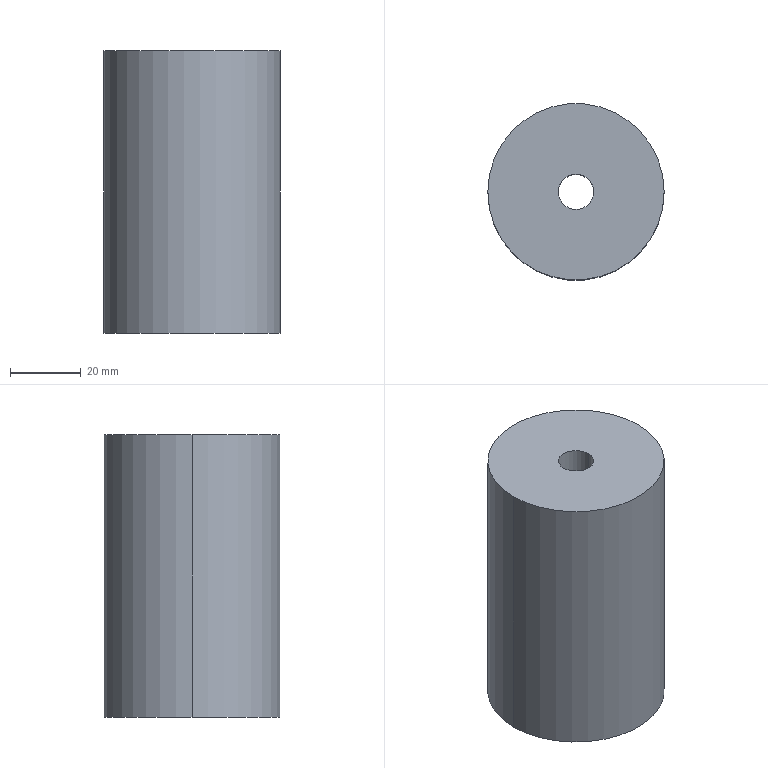Part | SolidWorks | features Extrusion 1 | 1 solid | 6 faces | box 50 x 50 x 80 mm | volume 150796 mm3 | cylinder 4 | plane 2 | commonest cylinder face diameters 10 x2 50 x2
STEP:
#1=CARTESIAN_POINT('',(-5.,0.,80.));
#2=VERTEX_POINT('',#1);
#3=CARTESIAN_POINT('',(5.,0.,80.));
#4=VERTEX_POINT('',#3);
#5=CARTESIAN_POINT('',(0.,0.,80.));
#6=DIRECTION('',(0.,0.,1.));
#7=DIRECTION('',(1.,0.,0.));
#8=AXIS2_PLACEMENT_3D('',#5,#6,#7);
#9=CIRCLE('',#8,5.);
#10=EDGE_CURVE('',#2,#4,#9,.T.);
#11=ORIENTED_EDGE('',*,*,#10,.T.);
#12=CARTESIAN_POINT('',(5.,0.,0.));
#13=VERTEX_POINT('',#12);
#14=CARTESIAN_POINT('',(5.,0.,80.));
#15=DIRECTION('',(0.,0.,-1.));
#16=VECTOR('',#15,1000.);
#17=LINE('',#14,#16);
#18=EDGE_CURVE('',#4,#13,#17,.T.);
#19=ORIENTED_EDGE('',*,*,#18,.T.);
#20=CARTESIAN_POINT('',(-5.,0.,0.));
#21=VERTEX_POINT('',#20);
#22=CARTESIAN_POINT('',(0.,0.,0.));
#23=DIRECTION('',(0.,0.,1.));
#24=DIRECTION('',(1.,0.,0.));
#25=AXIS2_PLACEMENT_3D('',#22,#23,#24);
#26=CIRCLE('',#25,5.);
#27=EDGE_CURVE('',#21,#13,#26,.T.);
#28=ORIENTED_EDGE('',*,*,#27,.F.);
#29=CARTESIAN_POINT('',(-5.,0.,80.));
#30=DIRECTION('',(0.,0.,-1.));
#31=VECTOR('',#30,1000.);
#32=LINE('',#29,#31);
#33=EDGE_CURVE('',#2,#21,#32,.T.);
#34=ORIENTED_EDGE('',*,*,#33,.F.);
#35=EDGE_LOOP('',(#11,#19,#28,#34));
#36=FACE_OUTER_BOUND('',#35,.T.);
#37=CARTESIAN_POINT('',(0.,0.,80.));
#38=DIRECTION('',(0.,0.,-1.));
#39=DIRECTION('',(-1.,0.,0.));
#40=AXIS2_PLACEMENT_3D('',#37,#38,#39);
#41=CYLINDRICAL_SURFACE('',#40,5.);
#42=ADVANCED_FACE('',(#36),#41,.F.);
#43=CARTESIAN_POINT('',(25.,0.,80.));
#44=VERTEX_POINT('',#43);
#45=CARTESIAN_POINT('',(-25.,0.,80.));
#46=VERTEX_POINT('',#45);
#47=CARTESIAN_POINT('',(0.,0.,80.));
#48=DIRECTION('',(0.,0.,1.));
#49=DIRECTION('',(1.,0.,0.));
#50=AXIS2_PLACEMENT_3D('',#47,#48,#49);
#51=CIRCLE('',#50,25.);
#52=EDGE_CURVE('',#44,#46,#51,.T.);
#53=ORIENTED_EDGE('',*,*,#52,.F.);
#54=CARTESIAN_POINT('',(25.,0.,0.));
#55=VERTEX_POINT('',#54);
#56=CARTESIAN_POINT('',(25.,0.,80.));
#57=DIRECTION('',(0.,0.,-1.));
#58=VECTOR('',#57,1000.);
#59=LINE('',#56,#58);
#60=EDGE_CURVE('',#44,#55,#59,.T.);
#61=ORIENTED_EDGE('',*,*,#60,.T.);
#62=CARTESIAN_POINT('',(-25.,0.,0.));
#63=VERTEX_POINT('',#62);
#64=CARTESIAN_POINT('',(0.,0.,0.));
#65=DIRECTION('',(0.,0.,1.));
#66=DIRECTION('',(1.,0.,0.));
#67=AXIS2_PLACEMENT_3D('',#64,#65,#66);
#68=CIRCLE('',#67,25.);
#69=EDGE_CURVE('',#55,#63,#68,.T.);
#70=ORIENTED_EDGE('',*,*,#69,.T.);
#71=CARTESIAN_POINT('',(-25.,0.,80.));
#72=DIRECTION('',(0.,0.,-1.));
#73=VECTOR('',#72,1000.);
#74=LINE('',#71,#73);
#75=EDGE_CURVE('',#46,#63,#74,.T.);
#76=ORIENTED_EDGE('',*,*,#75,.F.);
#77=EDGE_LOOP('',(#53,#61,#70,#76));
#78=FACE_OUTER_BOUND('',#77,.T.);
#79=CARTESIAN_POINT('',(0.,0.,80.));
#80=DIRECTION('',(0.,0.,-1.));
#81=DIRECTION('',(-1.,0.,0.));
#82=AXIS2_PLACEMENT_3D('',#79,#80,#81);
#83=CYLINDRICAL_SURFACE('',#82,25.);
#84=ADVANCED_FACE('',(#78),#83,.T.);
#85=CARTESIAN_POINT('',(0.,0.,80.));
#86=DIRECTION('',(0.,0.,1.));
#87=DIRECTION('',(1.,0.,0.));
#88=AXIS2_PLACEMENT_3D('',#85,#86,#87);
#89=CIRCLE('',#88,25.);
#90=EDGE_CURVE('',#46,#44,#89,.T.);
#91=ORIENTED_EDGE('',*,*,#90,.T.);
#92=ORIENTED_EDGE('',*,*,#52,.T.);
#93=EDGE_LOOP('',(#91,#92));
#94=FACE_OUTER_BOUND('',#93,.T.);
#95=ORIENTED_EDGE('',*,*,#10,.F.);
#96=CARTESIAN_POINT('',(0.,0.,80.));
#97=DIRECTION('',(0.,0.,1.));
#98=DIRECTION('',(1.,0.,0.));
#99=AXIS2_PLACEMENT_3D('',#96,#97,#98);
#100=CIRCLE('',#99,5.);
#101=EDGE_CURVE('',#4,#2,#100,.T.);
#102=ORIENTED_EDGE('',*,*,#101,.F.);
#103=EDGE_LOOP('',(#95,#102));
#104=FACE_BOUND('',#103,.T.);
#105=CARTESIAN_POINT('',(0.,0.,80.));
#106=DIRECTION('',(0.,0.,1.));
#107=DIRECTION('',(1.,0.,0.));
#108=AXIS2_PLACEMENT_3D('',#105,#106,#107);
#109=PLANE('',#108);
#110=ADVANCED_FACE('',(#94,#104),#109,.T.);
#111=CARTESIAN_POINT('',(0.,0.,0.));
#112=DIRECTION('',(0.,0.,1.));
#113=DIRECTION('',(1.,0.,0.));
#114=AXIS2_PLACEMENT_3D('',#111,#112,#113);
#115=CIRCLE('',#114,25.);
#116=EDGE_CURVE('',#63,#55,#115,.T.);
#117=ORIENTED_EDGE('',*,*,#116,.F.);
#118=ORIENTED_EDGE('',*,*,#69,.F.);
#119=EDGE_LOOP('',(#117,#118));
#120=FACE_OUTER_BOUND('',#119,.T.);
#121=ORIENTED_EDGE('',*,*,#27,.T.);
#122=CARTESIAN_POINT('',(0.,0.,0.));
#123=DIRECTION('',(0.,0.,1.));
#124=DIRECTION('',(1.,0.,0.));
#125=AXIS2_PLACEMENT_3D('',#122,#123,#124);
#126=CIRCLE('',#125,5.);
#127=EDGE_CURVE('',#13,#21,#126,.T.);
#128=ORIENTED_EDGE('',*,*,#127,.T.);
#129=EDGE_LOOP('',(#121,#128));
#130=FACE_BOUND('',#129,.T.);
#131=CARTESIAN_POINT('',(0.,0.,0.));
#132=DIRECTION('',(0.,0.,1.));
#133=DIRECTION('',(1.,0.,0.));
#134=AXIS2_PLACEMENT_3D('',#131,#132,#133);
#135=PLANE('',#134);
#136=ADVANCED_FACE('',(#120,#130),#135,.F.);
#137=ORIENTED_EDGE('',*,*,#60,.F.);
#138=ORIENTED_EDGE('',*,*,#90,.F.);
#139=ORIENTED_EDGE('',*,*,#75,.T.);
#140=ORIENTED_EDGE('',*,*,#116,.T.);
#141=EDGE_LOOP('',(#137,#138,#139,#140));
#142=FACE_OUTER_BOUND('',#141,.T.);
#143=CARTESIAN_POINT('',(0.,0.,80.));
#144=DIRECTION('',(0.,0.,-1.));
#145=DIRECTION('',(-1.,0.,0.));
#146=AXIS2_PLACEMENT_3D('',#143,#144,#145);
#147=CYLINDRICAL_SURFACE('',#146,25.);
#148=ADVANCED_FACE('',(#142),#147,.T.);
#149=ORIENTED_EDGE('',*,*,#18,.F.);
#150=ORIENTED_EDGE('',*,*,#101,.T.);
#151=ORIENTED_EDGE('',*,*,#33,.T.);
#152=ORIENTED_EDGE('',*,*,#127,.F.);
#153=EDGE_LOOP('',(#149,#150,#151,#152));
#154=FACE_OUTER_BOUND('',#153,.T.);
#155=CARTESIAN_POINT('',(0.,0.,80.));
#156=DIRECTION('',(0.,0.,-1.));
#157=DIRECTION('',(-1.,0.,0.));
#158=AXIS2_PLACEMENT_3D('',#155,#156,#157);
#159=CYLINDRICAL_SURFACE('',#158,5.);
#160=ADVANCED_FACE('',(#154),#159,.F.);
#161=CLOSED_SHELL('',(#42,#84,#110,#136,#148,#160));
#162=MANIFOLD_SOLID_BREP('',#161);
#163=CARTESIAN_POINT('',(0.,0.,0.));
#164=DIRECTION('',(0.,0.,1.));
#165=DIRECTION('',(1.,0.,0.));
#166=AXIS2_PLACEMENT_3D('',#163,#164,#165);
#167=(LENGTH_UNIT()NAMED_UNIT(*)SI_UNIT(.MILLI.,.METRE.));
#168=UNCERTAINTY_MEASURE_WITH_UNIT(LENGTH_MEASURE(0.00001),#167,'','');
#169=(NAMED_UNIT(*)PLANE_ANGLE_UNIT()SI_UNIT($,.RADIAN.));
#170=(NAMED_UNIT(*)SI_UNIT($,.STERADIAN.)SOLID_ANGLE_UNIT());
#171=(GEOMETRIC_REPRESENTATION_CONTEXT(3)GLOBAL_UNCERTAINTY_ASSIGNED_CONTEXT((#168))GLOBAL_UNIT_ASSIGNED_CONTEXT((#167,#169,#170))REPRESENTATION_CONTEXT('',''));
#172=ADVANCED_BREP_SHAPE_REPRESENTATION('',(#162,#166),#171);